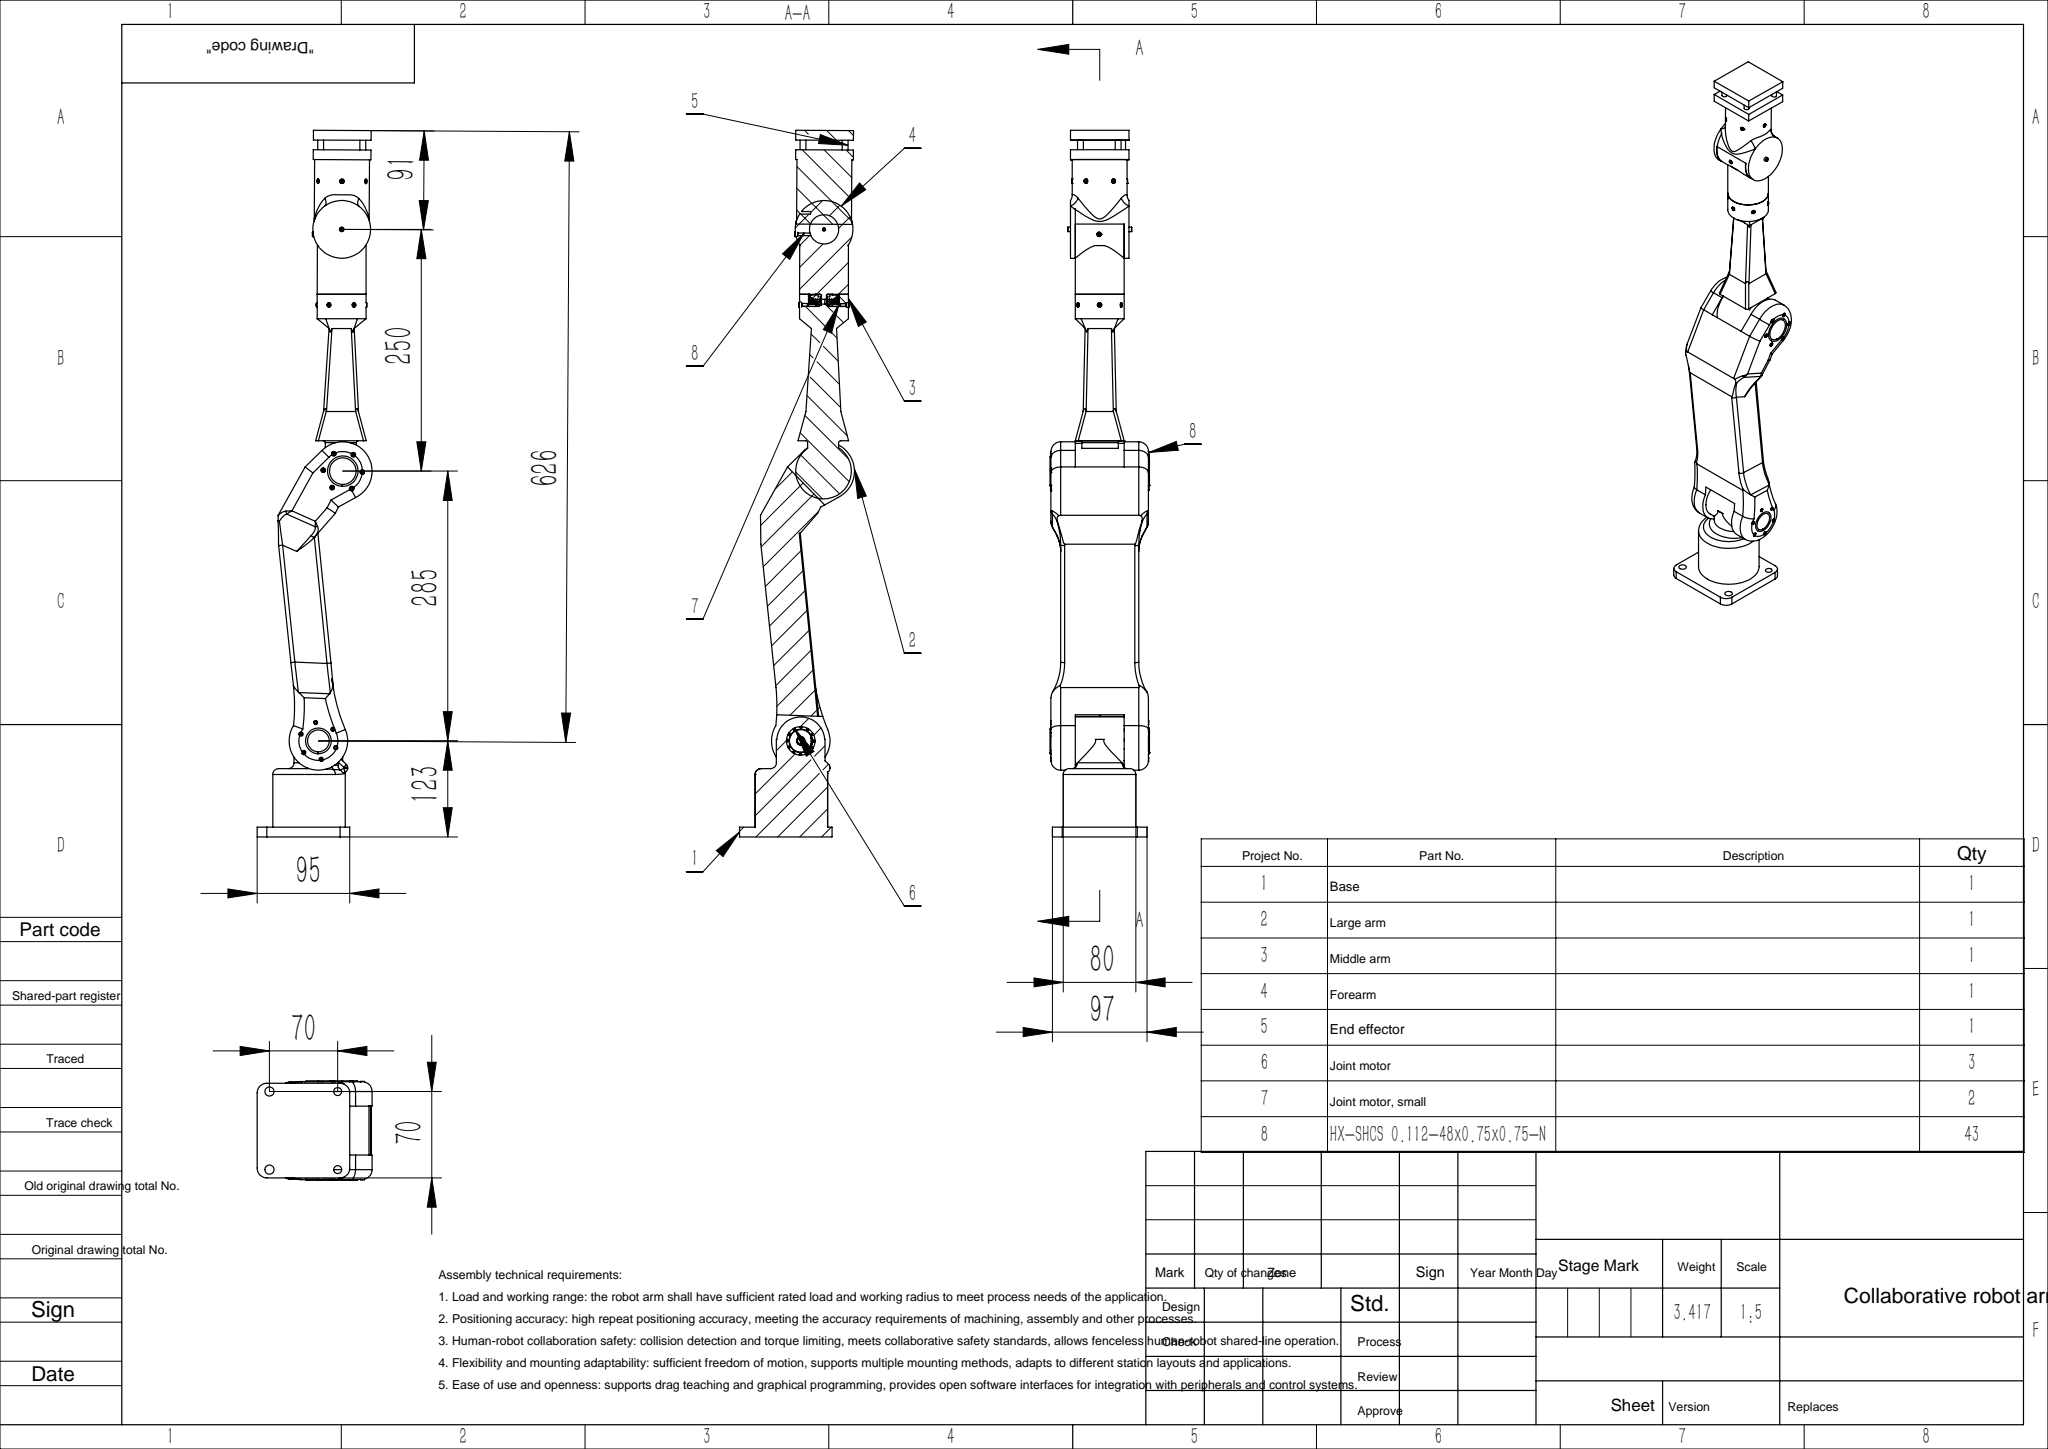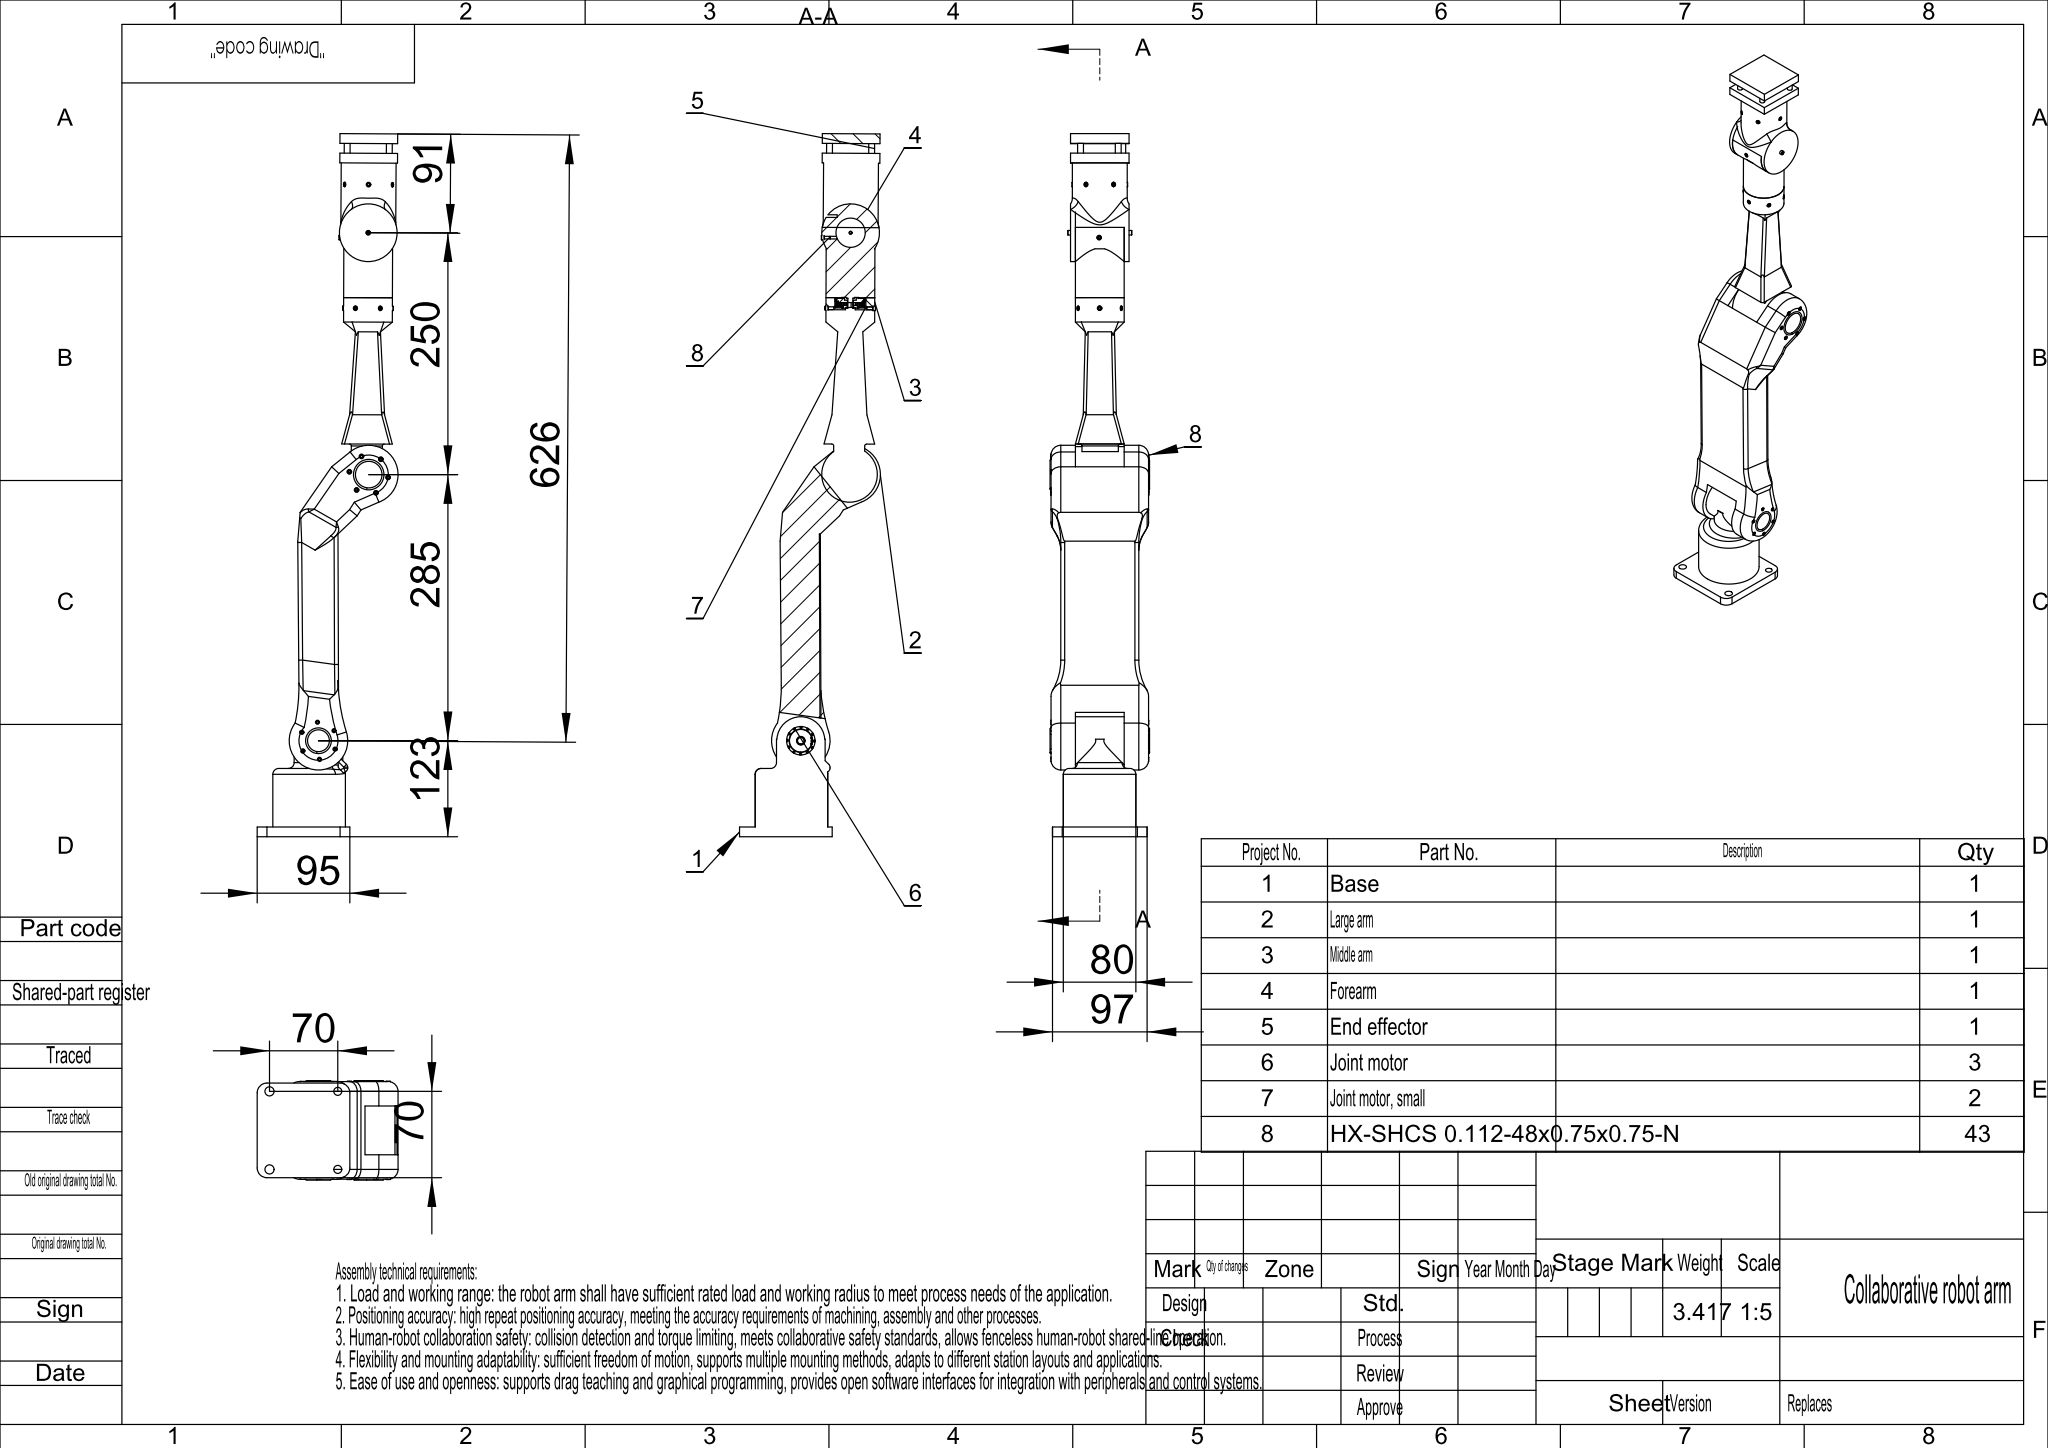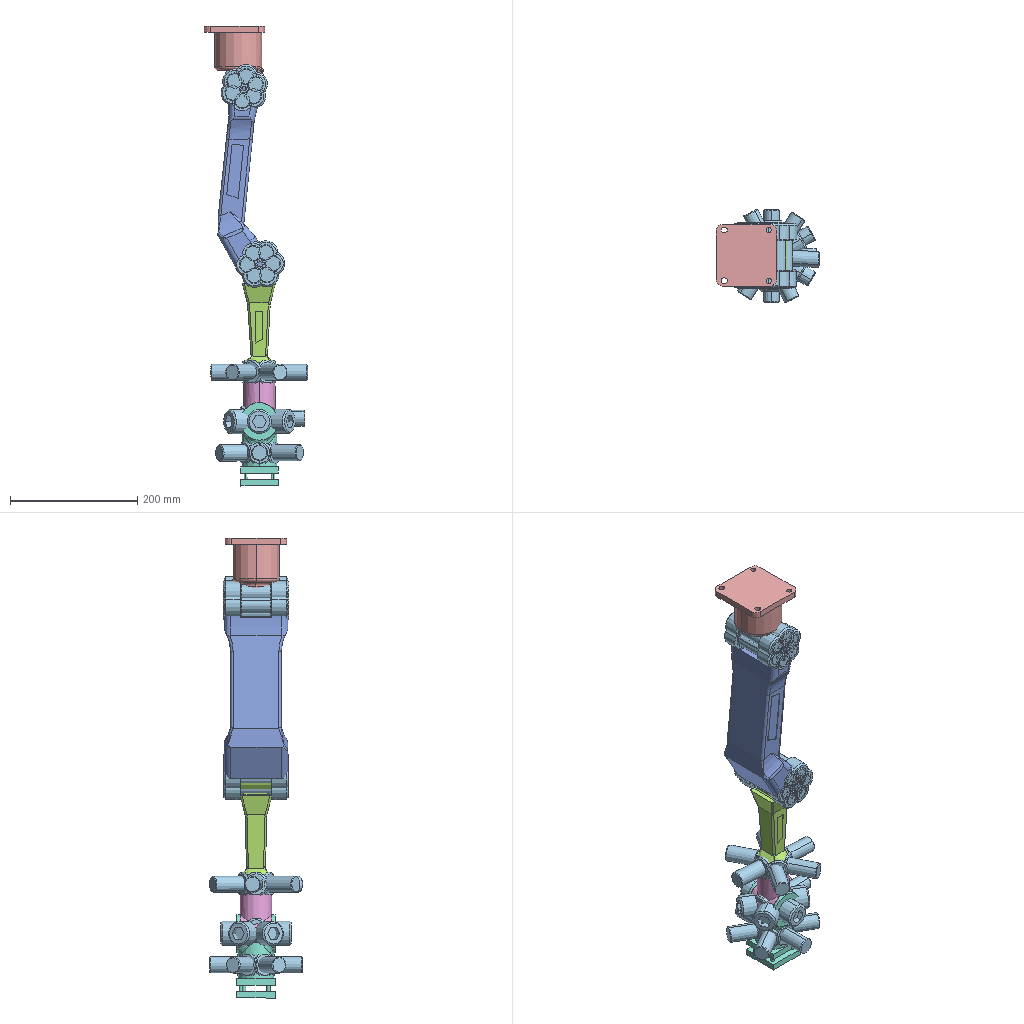Assembly | SolidWorks | 8 different items | 11 placed | box 163 x 147 x 724 mm
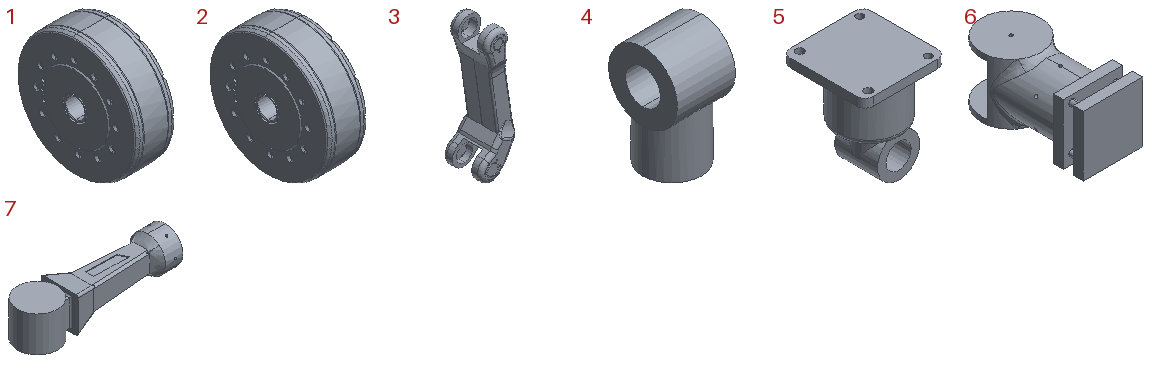Parts list (item | name | quantity | size | volume | features):
1 | - | x3 | 14.8 x 42.4 x 42.4 mm | 8202 mm3 | features BaseBody 3, ICE 1, Scale 1
2 | - | x2 | 11.1 x 31.8 x 31.8 mm | 3460 mm3 | features BaseBody 3, ICE 1, Scale 1
3 | - | x1 | 94.476 x 102 x 337.299 mm | 1069129 mm3 | features ICE 10, Fillet 7, CutThin 3, MirrorPattern 3, CirPattern 2, Sweep 2, Extrusion 1
4 | - | x1 | 50 x 59.155 x 101.162 mm | 183899 mm3 | features ICE 4, Extrusion 1, RefAxis 1
5 | - | x1 | 95 x 97 x 123 mm | 427032 mm3 | features Fillet 5, ICE 5, Extrusion 1
6 | - | x1 | 59.155 x 131.009 x 60 mm | 266464 mm3 | features ICE 5, CirPattern 1, CutThin 1, Extrusion 1, Fillet 1
7 | - | x1 | 209.608 x 56.982 x 50.008 mm | 324433 mm3 | features ICE 6, Blend 2, Fillet 2, Chamfer 1, CirPattern 1, Extrusion 1
8 | socket head cap screw_ai | x1 | - | - | -
Mates (type | each side: item.copy, entity, surface, feature):
Coincident | 5.1 face plane Boss-Extrude3 | 3.1 face plane Cut-Extrude-Thin1
Concentric | 3.1 face cylinder Boss-Extrude1 | 7.1 face cylinder Boss-Extrude1
Coincident | 3.1 face plane Cut-Extrude-Thin3 | 7.1 face plane Boss-Extrude1
Concentric | 7.1 face cylinder Cut-Extrude1 | 4.1 face cylinder Boss-Extrude3
Coincident | 7.1 face plane Boss-Extrude5 | 4.1 edge
Concentric | 4.1 face cylinder Boss-Extrude2 | 6.1 face cylinder Boss-Extrude1
Coincident | 4.1 face plane Boss-Extrude2 | 6.1 face plane Cut-Extrude-Thin1
Parallel | 3.1 face plane Boss-Extrude2 | 6.1 face plane Boss-Extrude1
Concentric | 3.1 face cylinder Cut-Extrude6 | 1.1 face cylinder 106 Assembly.STEP-1/106mm Drive and control one-piece motor.STEP-1-solid10
Coincident | 3.1 face plane Cut-Extrude-Thin1 | 1.1 face plane 106 Assembly.STEP-1/106mm Drive and control one-piece motor.STEP-1-solid10
Concentric | 3.1 face cylinder Cut-Extrude5 | 1.2 face cylinder 106 Assembly.STEP-1/106mm Drive and control one-piece motor.STEP-1-solid10
Coincident | 3.1 face plane Cut-Extrude-Thin1 | 1.2 face plane 106 Assembly.STEP-1/106mm Drive and control one-piece motor.STEP-1-solid12
Concentric | 3.1 face cylinder Boss-Extrude1 | 1.3 face cylinder 106 Assembly.STEP-1/106mm Drive and control one-piece motor.STEP-1-solid10
Coincident | 3.1 face plane Cut-Extrude-Thin3 | 1.3 face plane 106 Assembly.STEP-1/106mm Drive and control one-piece motor.STEP-1-solid12
Concentric | 7.1 face cylinder Cut-Extrude1 | 2.1 face cylinder 106 Assembly.STEP-1/106mm Drive and control one-piece motor.STEP-1-solid10
Coincident | 7.1 face plane Boss-Extrude5 | 2.1 face plane 106 Assembly.STEP-1/106mm Drive and control one-piece motor.STEP-1-solid10
Concentric | 4.1 face cylinder Cut-Extrude1 | 2.2 face cylinder 106 Assembly.STEP-1/106mm Drive and control one-piece motor.STEP-1-solid10
DistanceDim | 2.2 face plane 106 Assembly.STEP-1/106mm Drive and control one-piece motor.STEP-1-solid10 | 4.1 face plane Boss-Extrude2
Concentric | 5.1 face cylinder Cut-Extrude1 | 1.2 face cylinder 106 Assembly.STEP-1/106mm Drive and control one-piece motor.STEP-1-solid10